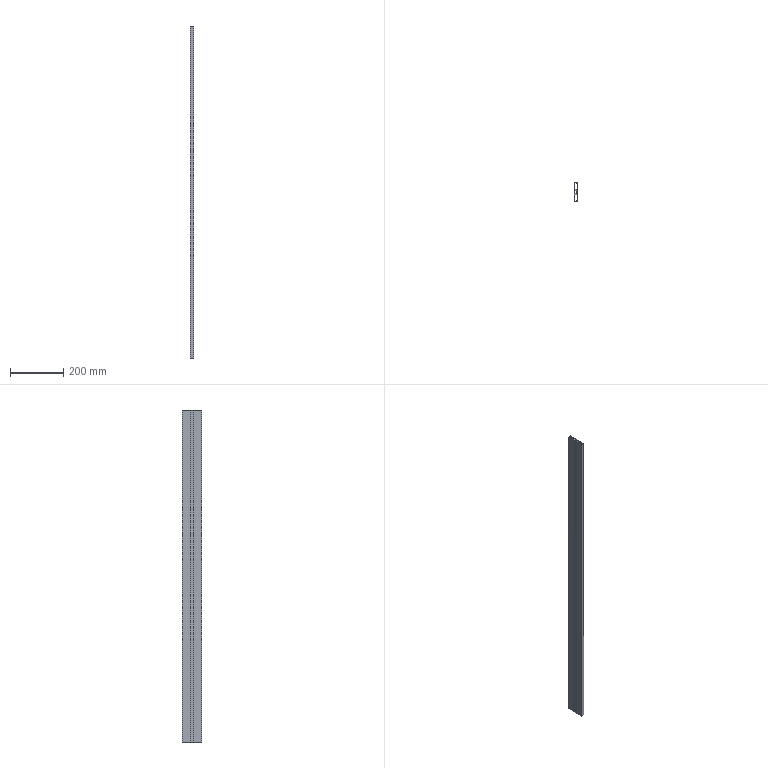Part | SolidWorks | features Extrusion 1 | 1 solid | 22 faces | box 12 x 73 x 1250 mm | volume 455000 mm3 | plane 22
STEP:
#1=CARTESIAN_POINT('',(-12.,36.5,625.));
#2=VERTEX_POINT('',#1);
#3=CARTESIAN_POINT('',(-12.,4.5,625.));
#4=VERTEX_POINT('',#3);
#5=CARTESIAN_POINT('',(-12.,36.5,625.));
#6=DIRECTION('',(0.,-1.,0.));
#7=VECTOR('',#6,1000.);
#8=LINE('',#5,#7);
#9=EDGE_CURVE('',#2,#4,#8,.T.);
#10=ORIENTED_EDGE('',*,*,#9,.T.);
#11=CARTESIAN_POINT('',(-10.,4.5,625.));
#12=VERTEX_POINT('',#11);
#13=CARTESIAN_POINT('',(-12.,4.5,625.));
#14=DIRECTION('',(1.,0.,0.));
#15=VECTOR('',#14,1000.);
#16=LINE('',#13,#15);
#17=EDGE_CURVE('',#4,#12,#16,.T.);
#18=ORIENTED_EDGE('',*,*,#17,.T.);
#19=CARTESIAN_POINT('',(-10.,6.5,625.));
#20=VERTEX_POINT('',#19);
#21=CARTESIAN_POINT('',(-10.,4.5,625.));
#22=DIRECTION('',(0.,1.,0.));
#23=VECTOR('',#22,1000.);
#24=LINE('',#21,#23);
#25=EDGE_CURVE('',#12,#20,#24,.T.);
#26=ORIENTED_EDGE('',*,*,#25,.T.);
#27=CARTESIAN_POINT('',(-4.,6.5,625.));
#28=VERTEX_POINT('',#27);
#29=CARTESIAN_POINT('',(-10.,6.5,625.));
#30=DIRECTION('',(1.,0.,0.));
#31=VECTOR('',#30,1000.);
#32=LINE('',#29,#31);
#33=EDGE_CURVE('',#20,#28,#32,.T.);
#34=ORIENTED_EDGE('',*,*,#33,.T.);
#35=CARTESIAN_POINT('',(-4.,-6.5,625.));
#36=VERTEX_POINT('',#35);
#37=CARTESIAN_POINT('',(-4.,6.5,625.));
#38=DIRECTION('',(0.,-1.,0.));
#39=VECTOR('',#38,1000.);
#40=LINE('',#37,#39);
#41=EDGE_CURVE('',#28,#36,#40,.T.);
#42=ORIENTED_EDGE('',*,*,#41,.T.);
#43=CARTESIAN_POINT('',(-10.,-6.5,625.));
#44=VERTEX_POINT('',#43);
#45=CARTESIAN_POINT('',(-4.,-6.5,625.));
#46=DIRECTION('',(-1.,0.,0.));
#47=VECTOR('',#46,1000.);
#48=LINE('',#45,#47);
#49=EDGE_CURVE('',#36,#44,#48,.T.);
#50=ORIENTED_EDGE('',*,*,#49,.T.);
#51=CARTESIAN_POINT('',(-10.,-4.5,625.));
#52=VERTEX_POINT('',#51);
#53=CARTESIAN_POINT('',(-10.,-6.5,625.));
#54=DIRECTION('',(0.,1.,0.));
#55=VECTOR('',#54,1000.);
#56=LINE('',#53,#55);
#57=EDGE_CURVE('',#44,#52,#56,.T.);
#58=ORIENTED_EDGE('',*,*,#57,.T.);
#59=CARTESIAN_POINT('',(-12.,-4.5,625.));
#60=VERTEX_POINT('',#59);
#61=CARTESIAN_POINT('',(-10.,-4.5,625.));
#62=DIRECTION('',(-1.,0.,0.));
#63=VECTOR('',#62,1000.);
#64=LINE('',#61,#63);
#65=EDGE_CURVE('',#52,#60,#64,.T.);
#66=ORIENTED_EDGE('',*,*,#65,.T.);
#67=CARTESIAN_POINT('',(-12.,-36.5,625.));
#68=VERTEX_POINT('',#67);
#69=CARTESIAN_POINT('',(-12.,-4.5,625.));
#70=DIRECTION('',(0.,-1.,0.));
#71=VECTOR('',#70,1000.);
#72=LINE('',#69,#71);
#73=EDGE_CURVE('',#60,#68,#72,.T.);
#74=ORIENTED_EDGE('',*,*,#73,.T.);
#75=CARTESIAN_POINT('',(0.,-36.5,625.));
#76=VERTEX_POINT('',#75);
#77=CARTESIAN_POINT('',(-12.,-36.5,625.));
#78=DIRECTION('',(1.,0.,0.));
#79=VECTOR('',#78,1000.);
#80=LINE('',#77,#79);
#81=EDGE_CURVE('',#68,#76,#80,.T.);
#82=ORIENTED_EDGE('',*,*,#81,.T.);
#83=CARTESIAN_POINT('',(0.,36.5,625.));
#84=VERTEX_POINT('',#83);
#85=CARTESIAN_POINT('',(0.,-36.5,625.));
#86=DIRECTION('',(0.,1.,0.));
#87=VECTOR('',#86,1000.);
#88=LINE('',#85,#87);
#89=EDGE_CURVE('',#76,#84,#88,.T.);
#90=ORIENTED_EDGE('',*,*,#89,.T.);
#91=CARTESIAN_POINT('',(0.,36.5,625.));
#92=DIRECTION('',(-1.,0.,0.));
#93=VECTOR('',#92,1000.);
#94=LINE('',#91,#93);
#95=EDGE_CURVE('',#84,#2,#94,.T.);
#96=ORIENTED_EDGE('',*,*,#95,.T.);
#97=EDGE_LOOP('',(#10,#18,#26,#34,#42,#50,#58,#66,#74,#82,#90,#96));
#98=FACE_OUTER_BOUND('',#97,.T.);
#99=CARTESIAN_POINT('',(-10.,-34.5,625.));
#100=VERTEX_POINT('',#99);
#101=CARTESIAN_POINT('',(-2.,-34.5,625.));
#102=VERTEX_POINT('',#101);
#103=CARTESIAN_POINT('',(-2.,-34.5,625.));
#104=DIRECTION('',(1.,0.,0.));
#105=VECTOR('',#104,1000.);
#106=LINE('',#103,#105);
#107=EDGE_CURVE('',#100,#102,#106,.T.);
#108=ORIENTED_EDGE('',*,*,#107,.F.);
#109=CARTESIAN_POINT('',(-10.,-8.5,625.));
#110=VERTEX_POINT('',#109);
#111=CARTESIAN_POINT('',(-10.,-34.5,625.));
#112=DIRECTION('',(0.,-1.,0.));
#113=VECTOR('',#112,1000.);
#114=LINE('',#111,#113);
#115=EDGE_CURVE('',#110,#100,#114,.T.);
#116=ORIENTED_EDGE('',*,*,#115,.F.);
#117=CARTESIAN_POINT('',(-2.,-8.5,625.));
#118=VERTEX_POINT('',#117);
#119=CARTESIAN_POINT('',(-10.,-8.5,625.));
#120=DIRECTION('',(-1.,0.,0.));
#121=VECTOR('',#120,1000.);
#122=LINE('',#119,#121);
#123=EDGE_CURVE('',#118,#110,#122,.T.);
#124=ORIENTED_EDGE('',*,*,#123,.F.);
#125=CARTESIAN_POINT('',(-2.,-8.5,625.));
#126=DIRECTION('',(0.,1.,0.));
#127=VECTOR('',#126,1000.);
#128=LINE('',#125,#127);
#129=EDGE_CURVE('',#102,#118,#128,.T.);
#130=ORIENTED_EDGE('',*,*,#129,.F.);
#131=EDGE_LOOP('',(#108,#116,#124,#130));
#132=FACE_BOUND('',#131,.T.);
#133=CARTESIAN_POINT('',(-10.,34.5,625.));
#134=VERTEX_POINT('',#133);
#135=CARTESIAN_POINT('',(-10.,8.5,625.));
#136=VERTEX_POINT('',#135);
#137=CARTESIAN_POINT('',(-10.,8.5,625.));
#138=DIRECTION('',(0.,-1.,0.));
#139=VECTOR('',#138,1000.);
#140=LINE('',#137,#139);
#141=EDGE_CURVE('',#134,#136,#140,.T.);
#142=ORIENTED_EDGE('',*,*,#141,.F.);
#143=CARTESIAN_POINT('',(-2.,34.5,625.));
#144=VERTEX_POINT('',#143);
#145=CARTESIAN_POINT('',(-10.,34.5,625.));
#146=DIRECTION('',(-1.,0.,0.));
#147=VECTOR('',#146,1000.);
#148=LINE('',#145,#147);
#149=EDGE_CURVE('',#144,#134,#148,.T.);
#150=ORIENTED_EDGE('',*,*,#149,.F.);
#151=CARTESIAN_POINT('',(-2.,8.5,625.));
#152=VERTEX_POINT('',#151);
#153=CARTESIAN_POINT('',(-2.,34.5,625.));
#154=DIRECTION('',(0.,1.,0.));
#155=VECTOR('',#154,1000.);
#156=LINE('',#153,#155);
#157=EDGE_CURVE('',#152,#144,#156,.T.);
#158=ORIENTED_EDGE('',*,*,#157,.F.);
#159=CARTESIAN_POINT('',(-2.,8.5,625.));
#160=DIRECTION('',(1.,0.,0.));
#161=VECTOR('',#160,1000.);
#162=LINE('',#159,#161);
#163=EDGE_CURVE('',#136,#152,#162,.T.);
#164=ORIENTED_EDGE('',*,*,#163,.F.);
#165=EDGE_LOOP('',(#142,#150,#158,#164));
#166=FACE_BOUND('',#165,.T.);
#167=CARTESIAN_POINT('',(0.,0.,625.));
#168=DIRECTION('',(0.,0.,1.));
#169=DIRECTION('',(1.,0.,0.));
#170=AXIS2_PLACEMENT_3D('',#167,#168,#169);
#171=PLANE('',#170);
#172=ADVANCED_FACE('',(#98,#132,#166),#171,.T.);
#173=CARTESIAN_POINT('',(-10.,-8.5,-625.));
#174=VERTEX_POINT('',#173);
#175=CARTESIAN_POINT('',(-10.,-34.5,-625.));
#176=VERTEX_POINT('',#175);
#177=CARTESIAN_POINT('',(-10.,-34.5,-625.));
#178=DIRECTION('',(0.,-1.,0.));
#179=VECTOR('',#178,1000.);
#180=LINE('',#177,#179);
#181=EDGE_CURVE('',#174,#176,#180,.T.);
#182=ORIENTED_EDGE('',*,*,#181,.T.);
#183=CARTESIAN_POINT('',(-2.,-34.5,-625.));
#184=VERTEX_POINT('',#183);
#185=CARTESIAN_POINT('',(-2.,-34.5,-625.));
#186=DIRECTION('',(1.,0.,0.));
#187=VECTOR('',#186,1000.);
#188=LINE('',#185,#187);
#189=EDGE_CURVE('',#176,#184,#188,.T.);
#190=ORIENTED_EDGE('',*,*,#189,.T.);
#191=CARTESIAN_POINT('',(-2.,-8.5,-625.));
#192=VERTEX_POINT('',#191);
#193=CARTESIAN_POINT('',(-2.,-8.5,-625.));
#194=DIRECTION('',(0.,1.,0.));
#195=VECTOR('',#194,1000.);
#196=LINE('',#193,#195);
#197=EDGE_CURVE('',#184,#192,#196,.T.);
#198=ORIENTED_EDGE('',*,*,#197,.T.);
#199=CARTESIAN_POINT('',(-10.,-8.5,-625.));
#200=DIRECTION('',(-1.,0.,0.));
#201=VECTOR('',#200,1000.);
#202=LINE('',#199,#201);
#203=EDGE_CURVE('',#192,#174,#202,.T.);
#204=ORIENTED_EDGE('',*,*,#203,.T.);
#205=EDGE_LOOP('',(#182,#190,#198,#204));
#206=FACE_BOUND('',#205,.T.);
#207=CARTESIAN_POINT('',(-12.,36.5,-625.));
#208=VERTEX_POINT('',#207);
#209=CARTESIAN_POINT('',(-12.,4.5,-625.));
#210=VERTEX_POINT('',#209);
#211=CARTESIAN_POINT('',(-12.,36.5,-625.));
#212=DIRECTION('',(0.,-1.,0.));
#213=VECTOR('',#212,1000.);
#214=LINE('',#211,#213);
#215=EDGE_CURVE('',#208,#210,#214,.T.);
#216=ORIENTED_EDGE('',*,*,#215,.F.);
#217=CARTESIAN_POINT('',(0.,36.5,-625.));
#218=VERTEX_POINT('',#217);
#219=CARTESIAN_POINT('',(0.,36.5,-625.));
#220=DIRECTION('',(-1.,0.,0.));
#221=VECTOR('',#220,1000.);
#222=LINE('',#219,#221);
#223=EDGE_CURVE('',#218,#208,#222,.T.);
#224=ORIENTED_EDGE('',*,*,#223,.F.);
#225=CARTESIAN_POINT('',(0.,-36.5,-625.));
#226=VERTEX_POINT('',#225);
#227=CARTESIAN_POINT('',(0.,-36.5,-625.));
#228=DIRECTION('',(0.,1.,0.));
#229=VECTOR('',#228,1000.);
#230=LINE('',#227,#229);
#231=EDGE_CURVE('',#226,#218,#230,.T.);
#232=ORIENTED_EDGE('',*,*,#231,.F.);
#233=CARTESIAN_POINT('',(-12.,-36.5,-625.));
#234=VERTEX_POINT('',#233);
#235=CARTESIAN_POINT('',(-12.,-36.5,-625.));
#236=DIRECTION('',(1.,0.,0.));
#237=VECTOR('',#236,1000.);
#238=LINE('',#235,#237);
#239=EDGE_CURVE('',#234,#226,#238,.T.);
#240=ORIENTED_EDGE('',*,*,#239,.F.);
#241=CARTESIAN_POINT('',(-12.,-4.5,-625.));
#242=VERTEX_POINT('',#241);
#243=CARTESIAN_POINT('',(-12.,-4.5,-625.));
#244=DIRECTION('',(0.,-1.,0.));
#245=VECTOR('',#244,1000.);
#246=LINE('',#243,#245);
#247=EDGE_CURVE('',#242,#234,#246,.T.);
#248=ORIENTED_EDGE('',*,*,#247,.F.);
#249=CARTESIAN_POINT('',(-10.,-4.5,-625.));
#250=VERTEX_POINT('',#249);
#251=CARTESIAN_POINT('',(-10.,-4.5,-625.));
#252=DIRECTION('',(-1.,0.,0.));
#253=VECTOR('',#252,1000.);
#254=LINE('',#251,#253);
#255=EDGE_CURVE('',#250,#242,#254,.T.);
#256=ORIENTED_EDGE('',*,*,#255,.F.);
#257=CARTESIAN_POINT('',(-10.,-6.5,-625.));
#258=VERTEX_POINT('',#257);
#259=CARTESIAN_POINT('',(-10.,-6.5,-625.));
#260=DIRECTION('',(0.,1.,0.));
#261=VECTOR('',#260,1000.);
#262=LINE('',#259,#261);
#263=EDGE_CURVE('',#258,#250,#262,.T.);
#264=ORIENTED_EDGE('',*,*,#263,.F.);
#265=CARTESIAN_POINT('',(-4.,-6.5,-625.));
#266=VERTEX_POINT('',#265);
#267=CARTESIAN_POINT('',(-4.,-6.5,-625.));
#268=DIRECTION('',(-1.,0.,0.));
#269=VECTOR('',#268,1000.);
#270=LINE('',#267,#269);
#271=EDGE_CURVE('',#266,#258,#270,.T.);
#272=ORIENTED_EDGE('',*,*,#271,.F.);
#273=CARTESIAN_POINT('',(-4.,6.5,-625.));
#274=VERTEX_POINT('',#273);
#275=CARTESIAN_POINT('',(-4.,6.5,-625.));
#276=DIRECTION('',(0.,-1.,0.));
#277=VECTOR('',#276,1000.);
#278=LINE('',#275,#277);
#279=EDGE_CURVE('',#274,#266,#278,.T.);
#280=ORIENTED_EDGE('',*,*,#279,.F.);
#281=CARTESIAN_POINT('',(-10.,6.5,-625.));
#282=VERTEX_POINT('',#281);
#283=CARTESIAN_POINT('',(-10.,6.5,-625.));
#284=DIRECTION('',(1.,0.,0.));
#285=VECTOR('',#284,1000.);
#286=LINE('',#283,#285);
#287=EDGE_CURVE('',#282,#274,#286,.T.);
#288=ORIENTED_EDGE('',*,*,#287,.F.);
#289=CARTESIAN_POINT('',(-10.,4.5,-625.));
#290=VERTEX_POINT('',#289);
#291=CARTESIAN_POINT('',(-10.,4.5,-625.));
#292=DIRECTION('',(0.,1.,0.));
#293=VECTOR('',#292,1000.);
#294=LINE('',#291,#293);
#295=EDGE_CURVE('',#290,#282,#294,.T.);
#296=ORIENTED_EDGE('',*,*,#295,.F.);
#297=CARTESIAN_POINT('',(-12.,4.5,-625.));
#298=DIRECTION('',(1.,0.,0.));
#299=VECTOR('',#298,1000.);
#300=LINE('',#297,#299);
#301=EDGE_CURVE('',#210,#290,#300,.T.);
#302=ORIENTED_EDGE('',*,*,#301,.F.);
#303=EDGE_LOOP('',(#216,#224,#232,#240,#248,#256,#264,#272,#280,#288,#296,#302));
#304=FACE_OUTER_BOUND('',#303,.T.);
#305=CARTESIAN_POINT('',(-2.,34.5,-625.));
#306=VERTEX_POINT('',#305);
#307=CARTESIAN_POINT('',(-10.,34.5,-625.));
#308=VERTEX_POINT('',#307);
#309=CARTESIAN_POINT('',(-10.,34.5,-625.));
#310=DIRECTION('',(-1.,0.,0.));
#311=VECTOR('',#310,1000.);
#312=LINE('',#309,#311);
#313=EDGE_CURVE('',#306,#308,#312,.T.);
#314=ORIENTED_EDGE('',*,*,#313,.T.);
#315=CARTESIAN_POINT('',(-10.,8.5,-625.));
#316=VERTEX_POINT('',#315);
#317=CARTESIAN_POINT('',(-10.,8.5,-625.));
#318=DIRECTION('',(0.,-1.,0.));
#319=VECTOR('',#318,1000.);
#320=LINE('',#317,#319);
#321=EDGE_CURVE('',#308,#316,#320,.T.);
#322=ORIENTED_EDGE('',*,*,#321,.T.);
#323=CARTESIAN_POINT('',(-2.,8.5,-625.));
#324=VERTEX_POINT('',#323);
#325=CARTESIAN_POINT('',(-2.,8.5,-625.));
#326=DIRECTION('',(1.,0.,0.));
#327=VECTOR('',#326,1000.);
#328=LINE('',#325,#327);
#329=EDGE_CURVE('',#316,#324,#328,.T.);
#330=ORIENTED_EDGE('',*,*,#329,.T.);
#331=CARTESIAN_POINT('',(-2.,34.5,-625.));
#332=DIRECTION('',(0.,1.,0.));
#333=VECTOR('',#332,1000.);
#334=LINE('',#331,#333);
#335=EDGE_CURVE('',#324,#306,#334,.T.);
#336=ORIENTED_EDGE('',*,*,#335,.T.);
#337=EDGE_LOOP('',(#314,#322,#330,#336));
#338=FACE_BOUND('',#337,.T.);
#339=CARTESIAN_POINT('',(0.,0.,-625.));
#340=DIRECTION('',(0.,0.,1.));
#341=DIRECTION('',(1.,0.,0.));
#342=AXIS2_PLACEMENT_3D('',#339,#340,#341);
#343=PLANE('',#342);
#344=ADVANCED_FACE('',(#206,#304,#338),#343,.F.);
#345=ORIENTED_EDGE('',*,*,#215,.T.);
#346=CARTESIAN_POINT('',(-12.,4.5,625.));
#347=DIRECTION('',(0.,0.,-1.));
#348=VECTOR('',#347,1000.);
#349=LINE('',#346,#348);
#350=EDGE_CURVE('',#4,#210,#349,.T.);
#351=ORIENTED_EDGE('',*,*,#350,.F.);
#352=ORIENTED_EDGE('',*,*,#9,.F.);
#353=CARTESIAN_POINT('',(-12.,36.5,625.));
#354=DIRECTION('',(0.,0.,-1.));
#355=VECTOR('',#354,1000.);
#356=LINE('',#353,#355);
#357=EDGE_CURVE('',#2,#208,#356,.T.);
#358=ORIENTED_EDGE('',*,*,#357,.T.);
#359=EDGE_LOOP('',(#345,#351,#352,#358));
#360=FACE_OUTER_BOUND('',#359,.T.);
#361=CARTESIAN_POINT('',(-12.,36.5,625.));
#362=DIRECTION('',(1.,0.,0.));
#363=DIRECTION('',(0.,0.,-1.));
#364=AXIS2_PLACEMENT_3D('',#361,#362,#363);
#365=PLANE('',#364);
#366=ADVANCED_FACE('',(#360),#365,.F.);
#367=ORIENTED_EDGE('',*,*,#301,.T.);
#368=CARTESIAN_POINT('',(-10.,4.5,625.));
#369=DIRECTION('',(0.,0.,-1.));
#370=VECTOR('',#369,1000.);
#371=LINE('',#368,#370);
#372=EDGE_CURVE('',#12,#290,#371,.T.);
#373=ORIENTED_EDGE('',*,*,#372,.F.);
#374=ORIENTED_EDGE('',*,*,#17,.F.);
#375=ORIENTED_EDGE('',*,*,#350,.T.);
#376=EDGE_LOOP('',(#367,#373,#374,#375));
#377=FACE_OUTER_BOUND('',#376,.T.);
#378=CARTESIAN_POINT('',(-12.,4.5,625.));
#379=DIRECTION('',(0.,1.,0.));
#380=DIRECTION('',(0.,0.,1.));
#381=AXIS2_PLACEMENT_3D('',#378,#379,#380);
#382=PLANE('',#381);
#383=ADVANCED_FACE('',(#377),#382,.F.);
#384=ORIENTED_EDGE('',*,*,#295,.T.);
#385=CARTESIAN_POINT('',(-10.,6.5,625.));
#386=DIRECTION('',(0.,0.,-1.));
#387=VECTOR('',#386,1000.);
#388=LINE('',#385,#387);
#389=EDGE_CURVE('',#20,#282,#388,.T.);
#390=ORIENTED_EDGE('',*,*,#389,.F.);
#391=ORIENTED_EDGE('',*,*,#25,.F.);
#392=ORIENTED_EDGE('',*,*,#372,.T.);
#393=EDGE_LOOP('',(#384,#390,#391,#392));
#394=FACE_OUTER_BOUND('',#393,.T.);
#395=CARTESIAN_POINT('',(-10.,4.5,625.));
#396=DIRECTION('',(-1.,0.,0.));
#397=DIRECTION('',(0.,0.,1.));
#398=AXIS2_PLACEMENT_3D('',#395,#396,#397);
#399=PLANE('',#398);
#400=ADVANCED_FACE('',(#394),#399,.F.);
#401=ORIENTED_EDGE('',*,*,#287,.T.);
#402=CARTESIAN_POINT('',(-4.,6.5,625.));
#403=DIRECTION('',(0.,0.,-1.));
#404=VECTOR('',#403,1000.);
#405=LINE('',#402,#404);
#406=EDGE_CURVE('',#28,#274,#405,.T.);
#407=ORIENTED_EDGE('',*,*,#406,.F.);
#408=ORIENTED_EDGE('',*,*,#33,.F.);
#409=ORIENTED_EDGE('',*,*,#389,.T.);
#410=EDGE_LOOP('',(#401,#407,#408,#409));
#411=FACE_OUTER_BOUND('',#410,.T.);
#412=CARTESIAN_POINT('',(-10.,6.5,625.));
#413=DIRECTION('',(0.,1.,0.));
#414=DIRECTION('',(0.,0.,1.));
#415=AXIS2_PLACEMENT_3D('',#412,#413,#414);
#416=PLANE('',#415);
#417=ADVANCED_FACE('',(#411),#416,.F.);
#418=ORIENTED_EDGE('',*,*,#279,.T.);
#419=CARTESIAN_POINT('',(-4.,-6.5,625.));
#420=DIRECTION('',(0.,0.,-1.));
#421=VECTOR('',#420,1000.);
#422=LINE('',#419,#421);
#423=EDGE_CURVE('',#36,#266,#422,.T.);
#424=ORIENTED_EDGE('',*,*,#423,.F.);
#425=ORIENTED_EDGE('',*,*,#41,.F.);
#426=ORIENTED_EDGE('',*,*,#406,.T.);
#427=EDGE_LOOP('',(#418,#424,#425,#426));
#428=FACE_OUTER_BOUND('',#427,.T.);
#429=CARTESIAN_POINT('',(-4.,6.5,625.));
#430=DIRECTION('',(1.,0.,0.));
#431=DIRECTION('',(0.,0.,-1.));
#432=AXIS2_PLACEMENT_3D('',#429,#430,#431);
#433=PLANE('',#432);
#434=ADVANCED_FACE('',(#428),#433,.F.);
#435=ORIENTED_EDGE('',*,*,#271,.T.);
#436=CARTESIAN_POINT('',(-10.,-6.5,625.));
#437=DIRECTION('',(0.,0.,-1.));
#438=VECTOR('',#437,1000.);
#439=LINE('',#436,#438);
#440=EDGE_CURVE('',#44,#258,#439,.T.);
#441=ORIENTED_EDGE('',*,*,#440,.F.);
#442=ORIENTED_EDGE('',*,*,#49,.F.);
#443=ORIENTED_EDGE('',*,*,#423,.T.);
#444=EDGE_LOOP('',(#435,#441,#442,#443));
#445=FACE_OUTER_BOUND('',#444,.T.);
#446=CARTESIAN_POINT('',(-4.,-6.5,625.));
#447=DIRECTION('',(0.,-1.,0.));
#448=DIRECTION('',(0.,0.,-1.));
#449=AXIS2_PLACEMENT_3D('',#446,#447,#448);
#450=PLANE('',#449);
#451=ADVANCED_FACE('',(#445),#450,.F.);
#452=ORIENTED_EDGE('',*,*,#263,.T.);
#453=CARTESIAN_POINT('',(-10.,-4.5,625.));
#454=DIRECTION('',(0.,0.,-1.));
#455=VECTOR('',#454,1000.);
#456=LINE('',#453,#455);
#457=EDGE_CURVE('',#52,#250,#456,.T.);
#458=ORIENTED_EDGE('',*,*,#457,.F.);
#459=ORIENTED_EDGE('',*,*,#57,.F.);
#460=ORIENTED_EDGE('',*,*,#440,.T.);
#461=EDGE_LOOP('',(#452,#458,#459,#460));
#462=FACE_OUTER_BOUND('',#461,.T.);
#463=CARTESIAN_POINT('',(-10.,-6.5,625.));
#464=DIRECTION('',(-1.,0.,0.));
#465=DIRECTION('',(0.,0.,1.));
#466=AXIS2_PLACEMENT_3D('',#463,#464,#465);
#467=PLANE('',#466);
#468=ADVANCED_FACE('',(#462),#467,.F.);
#469=ORIENTED_EDGE('',*,*,#255,.T.);
#470=CARTESIAN_POINT('',(-12.,-4.5,625.));
#471=DIRECTION('',(0.,0.,-1.));
#472=VECTOR('',#471,1000.);
#473=LINE('',#470,#472);
#474=EDGE_CURVE('',#60,#242,#473,.T.);
#475=ORIENTED_EDGE('',*,*,#474,.F.);
#476=ORIENTED_EDGE('',*,*,#65,.F.);
#477=ORIENTED_EDGE('',*,*,#457,.T.);
#478=EDGE_LOOP('',(#469,#475,#476,#477));
#479=FACE_OUTER_BOUND('',#478,.T.);
#480=CARTESIAN_POINT('',(-10.,-4.5,625.));
#481=DIRECTION('',(0.,-1.,0.));
#482=DIRECTION('',(0.,0.,-1.));
#483=AXIS2_PLACEMENT_3D('',#480,#481,#482);
#484=PLANE('',#483);
#485=ADVANCED_FACE('',(#479),#484,.F.);
#486=ORIENTED_EDGE('',*,*,#247,.T.);
#487=CARTESIAN_POINT('',(-12.,-36.5,625.));
#488=DIRECTION('',(0.,0.,-1.));
#489=VECTOR('',#488,1000.);
#490=LINE('',#487,#489);
#491=EDGE_CURVE('',#68,#234,#490,.T.);
#492=ORIENTED_EDGE('',*,*,#491,.F.);
#493=ORIENTED_EDGE('',*,*,#73,.F.);
#494=ORIENTED_EDGE('',*,*,#474,.T.);
#495=EDGE_LOOP('',(#486,#492,#493,#494));
#496=FACE_OUTER_BOUND('',#495,.T.);
#497=CARTESIAN_POINT('',(-12.,-4.5,625.));
#498=DIRECTION('',(1.,0.,0.));
#499=DIRECTION('',(0.,0.,-1.));
#500=AXIS2_PLACEMENT_3D('',#497,#498,#499);
#501=PLANE('',#500);
#502=ADVANCED_FACE('',(#496),#501,.F.);
#503=ORIENTED_EDGE('',*,*,#239,.T.);
#504=CARTESIAN_POINT('',(0.,-36.5,625.));
#505=DIRECTION('',(0.,0.,-1.));
#506=VECTOR('',#505,1000.);
#507=LINE('',#504,#506);
#508=EDGE_CURVE('',#76,#226,#507,.T.);
#509=ORIENTED_EDGE('',*,*,#508,.F.);
#510=ORIENTED_EDGE('',*,*,#81,.F.);
#511=ORIENTED_EDGE('',*,*,#491,.T.);
#512=EDGE_LOOP('',(#503,#509,#510,#511));
#513=FACE_OUTER_BOUND('',#512,.T.);
#514=CARTESIAN_POINT('',(-12.,-36.5,625.));
#515=DIRECTION('',(0.,1.,0.));
#516=DIRECTION('',(0.,0.,1.));
#517=AXIS2_PLACEMENT_3D('',#514,#515,#516);
#518=PLANE('',#517);
#519=ADVANCED_FACE('',(#513),#518,.F.);
#520=ORIENTED_EDGE('',*,*,#231,.T.);
#521=CARTESIAN_POINT('',(0.,36.5,625.));
#522=DIRECTION('',(0.,0.,-1.));
#523=VECTOR('',#522,1000.);
#524=LINE('',#521,#523);
#525=EDGE_CURVE('',#84,#218,#524,.T.);
#526=ORIENTED_EDGE('',*,*,#525,.F.);
#527=ORIENTED_EDGE('',*,*,#89,.F.);
#528=ORIENTED_EDGE('',*,*,#508,.T.);
#529=EDGE_LOOP('',(#520,#526,#527,#528));
#530=FACE_OUTER_BOUND('',#529,.T.);
#531=CARTESIAN_POINT('',(0.,-36.5,625.));
#532=DIRECTION('',(-1.,0.,0.));
#533=DIRECTION('',(0.,0.,1.));
#534=AXIS2_PLACEMENT_3D('',#531,#532,#533);
#535=PLANE('',#534);
#536=ADVANCED_FACE('',(#530),#535,.F.);
#537=ORIENTED_EDGE('',*,*,#223,.T.);
#538=ORIENTED_EDGE('',*,*,#357,.F.);
#539=ORIENTED_EDGE('',*,*,#95,.F.);
#540=ORIENTED_EDGE('',*,*,#525,.T.);
#541=EDGE_LOOP('',(#537,#538,#539,#540));
#542=FACE_OUTER_BOUND('',#541,.T.);
#543=CARTESIAN_POINT('',(0.,36.5,625.));
#544=DIRECTION('',(0.,-1.,0.));
#545=DIRECTION('',(0.,0.,-1.));
#546=AXIS2_PLACEMENT_3D('',#543,#544,#545);
#547=PLANE('',#546);
#548=ADVANCED_FACE('',(#542),#547,.F.);
#549=ORIENTED_EDGE('',*,*,#181,.F.);
#550=CARTESIAN_POINT('',(-10.,-8.5,625.));
#551=DIRECTION('',(0.,0.,-1.));
#552=VECTOR('',#551,1000.);
#553=LINE('',#550,#552);
#554=EDGE_CURVE('',#110,#174,#553,.T.);
#555=ORIENTED_EDGE('',*,*,#554,.F.);
#556=ORIENTED_EDGE('',*,*,#115,.T.);
#557=CARTESIAN_POINT('',(-10.,-34.5,625.));
#558=DIRECTION('',(0.,0.,-1.));
#559=VECTOR('',#558,1000.);
#560=LINE('',#557,#559);
#561=EDGE_CURVE('',#100,#176,#560,.T.);
#562=ORIENTED_EDGE('',*,*,#561,.T.);
#563=EDGE_LOOP('',(#549,#555,#556,#562));
#564=FACE_OUTER_BOUND('',#563,.T.);
#565=CARTESIAN_POINT('',(-10.,-34.5,625.));
#566=DIRECTION('',(1.,0.,0.));
#567=DIRECTION('',(0.,0.,-1.));
#568=AXIS2_PLACEMENT_3D('',#565,#566,#567);
#569=PLANE('',#568);
#570=ADVANCED_FACE('',(#564),#569,.T.);
#571=ORIENTED_EDGE('',*,*,#189,.F.);
#572=ORIENTED_EDGE('',*,*,#561,.F.);
#573=ORIENTED_EDGE('',*,*,#107,.T.);
#574=CARTESIAN_POINT('',(-2.,-34.5,625.));
#575=DIRECTION('',(0.,0.,-1.));
#576=VECTOR('',#575,1000.);
#577=LINE('',#574,#576);
#578=EDGE_CURVE('',#102,#184,#577,.T.);
#579=ORIENTED_EDGE('',*,*,#578,.T.);
#580=EDGE_LOOP('',(#571,#572,#573,#579));
#581=FACE_OUTER_BOUND('',#580,.T.);
#582=CARTESIAN_POINT('',(-2.,-34.5,625.));
#583=DIRECTION('',(0.,1.,0.));
#584=DIRECTION('',(0.,0.,1.));
#585=AXIS2_PLACEMENT_3D('',#582,#583,#584);
#586=PLANE('',#585);
#587=ADVANCED_FACE('',(#581),#586,.T.);
#588=ORIENTED_EDGE('',*,*,#197,.F.);
#589=ORIENTED_EDGE('',*,*,#578,.F.);
#590=ORIENTED_EDGE('',*,*,#129,.T.);
#591=CARTESIAN_POINT('',(-2.,-8.5,625.));
#592=DIRECTION('',(0.,0.,-1.));
#593=VECTOR('',#592,1000.);
#594=LINE('',#591,#593);
#595=EDGE_CURVE('',#118,#192,#594,.T.);
#596=ORIENTED_EDGE('',*,*,#595,.T.);
#597=EDGE_LOOP('',(#588,#589,#590,#596));
#598=FACE_OUTER_BOUND('',#597,.T.);
#599=CARTESIAN_POINT('',(-2.,-8.5,625.));
#600=DIRECTION('',(-1.,0.,0.));
#601=DIRECTION('',(0.,0.,1.));
#602=AXIS2_PLACEMENT_3D('',#599,#600,#601);
#603=PLANE('',#602);
#604=ADVANCED_FACE('',(#598),#603,.T.);
#605=ORIENTED_EDGE('',*,*,#203,.F.);
#606=ORIENTED_EDGE('',*,*,#595,.F.);
#607=ORIENTED_EDGE('',*,*,#123,.T.);
#608=ORIENTED_EDGE('',*,*,#554,.T.);
#609=EDGE_LOOP('',(#605,#606,#607,#608));
#610=FACE_OUTER_BOUND('',#609,.T.);
#611=CARTESIAN_POINT('',(-10.,-8.5,625.));
#612=DIRECTION('',(0.,-1.,0.));
#613=DIRECTION('',(0.,0.,-1.));
#614=AXIS2_PLACEMENT_3D('',#611,#612,#613);
#615=PLANE('',#614);
#616=ADVANCED_FACE('',(#610),#615,.T.);
#617=ORIENTED_EDGE('',*,*,#313,.F.);
#618=CARTESIAN_POINT('',(-2.,34.5,625.));
#619=DIRECTION('',(0.,0.,-1.));
#620=VECTOR('',#619,1000.);
#621=LINE('',#618,#620);
#622=EDGE_CURVE('',#144,#306,#621,.T.);
#623=ORIENTED_EDGE('',*,*,#622,.F.);
#624=ORIENTED_EDGE('',*,*,#149,.T.);
#625=CARTESIAN_POINT('',(-10.,34.5,625.));
#626=DIRECTION('',(0.,0.,-1.));
#627=VECTOR('',#626,1000.);
#628=LINE('',#625,#627);
#629=EDGE_CURVE('',#134,#308,#628,.T.);
#630=ORIENTED_EDGE('',*,*,#629,.T.);
#631=EDGE_LOOP('',(#617,#623,#624,#630));
#632=FACE_OUTER_BOUND('',#631,.T.);
#633=CARTESIAN_POINT('',(-10.,34.5,625.));
#634=DIRECTION('',(0.,-1.,0.));
#635=DIRECTION('',(0.,0.,-1.));
#636=AXIS2_PLACEMENT_3D('',#633,#634,#635);
#637=PLANE('',#636);
#638=ADVANCED_FACE('',(#632),#637,.T.);
#639=ORIENTED_EDGE('',*,*,#321,.F.);
#640=ORIENTED_EDGE('',*,*,#629,.F.);
#641=ORIENTED_EDGE('',*,*,#141,.T.);
#642=CARTESIAN_POINT('',(-10.,8.5,625.));
#643=DIRECTION('',(0.,0.,-1.));
#644=VECTOR('',#643,1000.);
#645=LINE('',#642,#644);
#646=EDGE_CURVE('',#136,#316,#645,.T.);
#647=ORIENTED_EDGE('',*,*,#646,.T.);
#648=EDGE_LOOP('',(#639,#640,#641,#647));
#649=FACE_OUTER_BOUND('',#648,.T.);
#650=CARTESIAN_POINT('',(-10.,8.5,625.));
#651=DIRECTION('',(1.,0.,0.));
#652=DIRECTION('',(0.,0.,-1.));
#653=AXIS2_PLACEMENT_3D('',#650,#651,#652);
#654=PLANE('',#653);
#655=ADVANCED_FACE('',(#649),#654,.T.);
#656=ORIENTED_EDGE('',*,*,#329,.F.);
#657=ORIENTED_EDGE('',*,*,#646,.F.);
#658=ORIENTED_EDGE('',*,*,#163,.T.);
#659=CARTESIAN_POINT('',(-2.,8.5,625.));
#660=DIRECTION('',(0.,0.,-1.));
#661=VECTOR('',#660,1000.);
#662=LINE('',#659,#661);
#663=EDGE_CURVE('',#152,#324,#662,.T.);
#664=ORIENTED_EDGE('',*,*,#663,.T.);
#665=EDGE_LOOP('',(#656,#657,#658,#664));
#666=FACE_OUTER_BOUND('',#665,.T.);
#667=CARTESIAN_POINT('',(-2.,8.5,625.));
#668=DIRECTION('',(0.,1.,0.));
#669=DIRECTION('',(0.,0.,1.));
#670=AXIS2_PLACEMENT_3D('',#667,#668,#669);
#671=PLANE('',#670);
#672=ADVANCED_FACE('',(#666),#671,.T.);
#673=ORIENTED_EDGE('',*,*,#335,.F.);
#674=ORIENTED_EDGE('',*,*,#663,.F.);
#675=ORIENTED_EDGE('',*,*,#157,.T.);
#676=ORIENTED_EDGE('',*,*,#622,.T.);
#677=EDGE_LOOP('',(#673,#674,#675,#676));
#678=FACE_OUTER_BOUND('',#677,.T.);
#679=CARTESIAN_POINT('',(-2.,34.5,625.));
#680=DIRECTION('',(-1.,0.,0.));
#681=DIRECTION('',(0.,0.,1.));
#682=AXIS2_PLACEMENT_3D('',#679,#680,#681);
#683=PLANE('',#682);
#684=ADVANCED_FACE('',(#678),#683,.T.);
#685=CLOSED_SHELL('',(#172,#344,#366,#383,#400,#417,#434,#451,#468,#485,#502,#519,#536,#548,#570,#587,#604,#616,#638,#655,#672,#684));
#686=MANIFOLD_SOLID_BREP('',#685);
#687=CARTESIAN_POINT('',(0.,0.,0.));
#688=DIRECTION('',(0.,0.,1.));
#689=DIRECTION('',(1.,0.,0.));
#690=AXIS2_PLACEMENT_3D('',#687,#688,#689);
#691=(LENGTH_UNIT()NAMED_UNIT(*)SI_UNIT(.MILLI.,.METRE.));
#692=UNCERTAINTY_MEASURE_WITH_UNIT(LENGTH_MEASURE(0.00001),#691,'','');
#693=(NAMED_UNIT(*)PLANE_ANGLE_UNIT()SI_UNIT($,.RADIAN.));
#694=(NAMED_UNIT(*)SI_UNIT($,.STERADIAN.)SOLID_ANGLE_UNIT());
#695=(GEOMETRIC_REPRESENTATION_CONTEXT(3)GLOBAL_UNCERTAINTY_ASSIGNED_CONTEXT((#692))GLOBAL_UNIT_ASSIGNED_CONTEXT((#691,#693,#694))REPRESENTATION_CONTEXT('',''));
#696=ADVANCED_BREP_SHAPE_REPRESENTATION('',(#686,#690),#695);